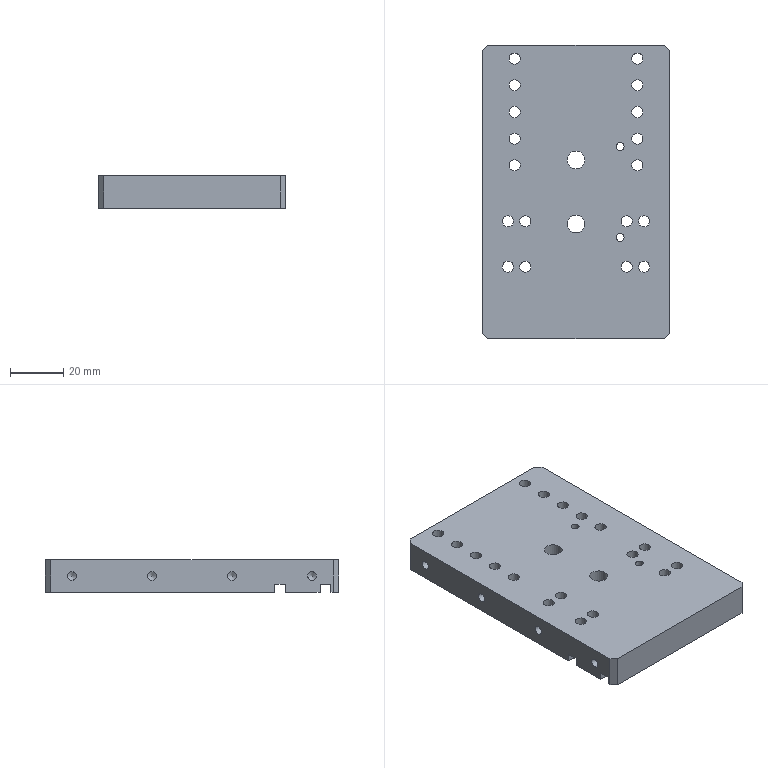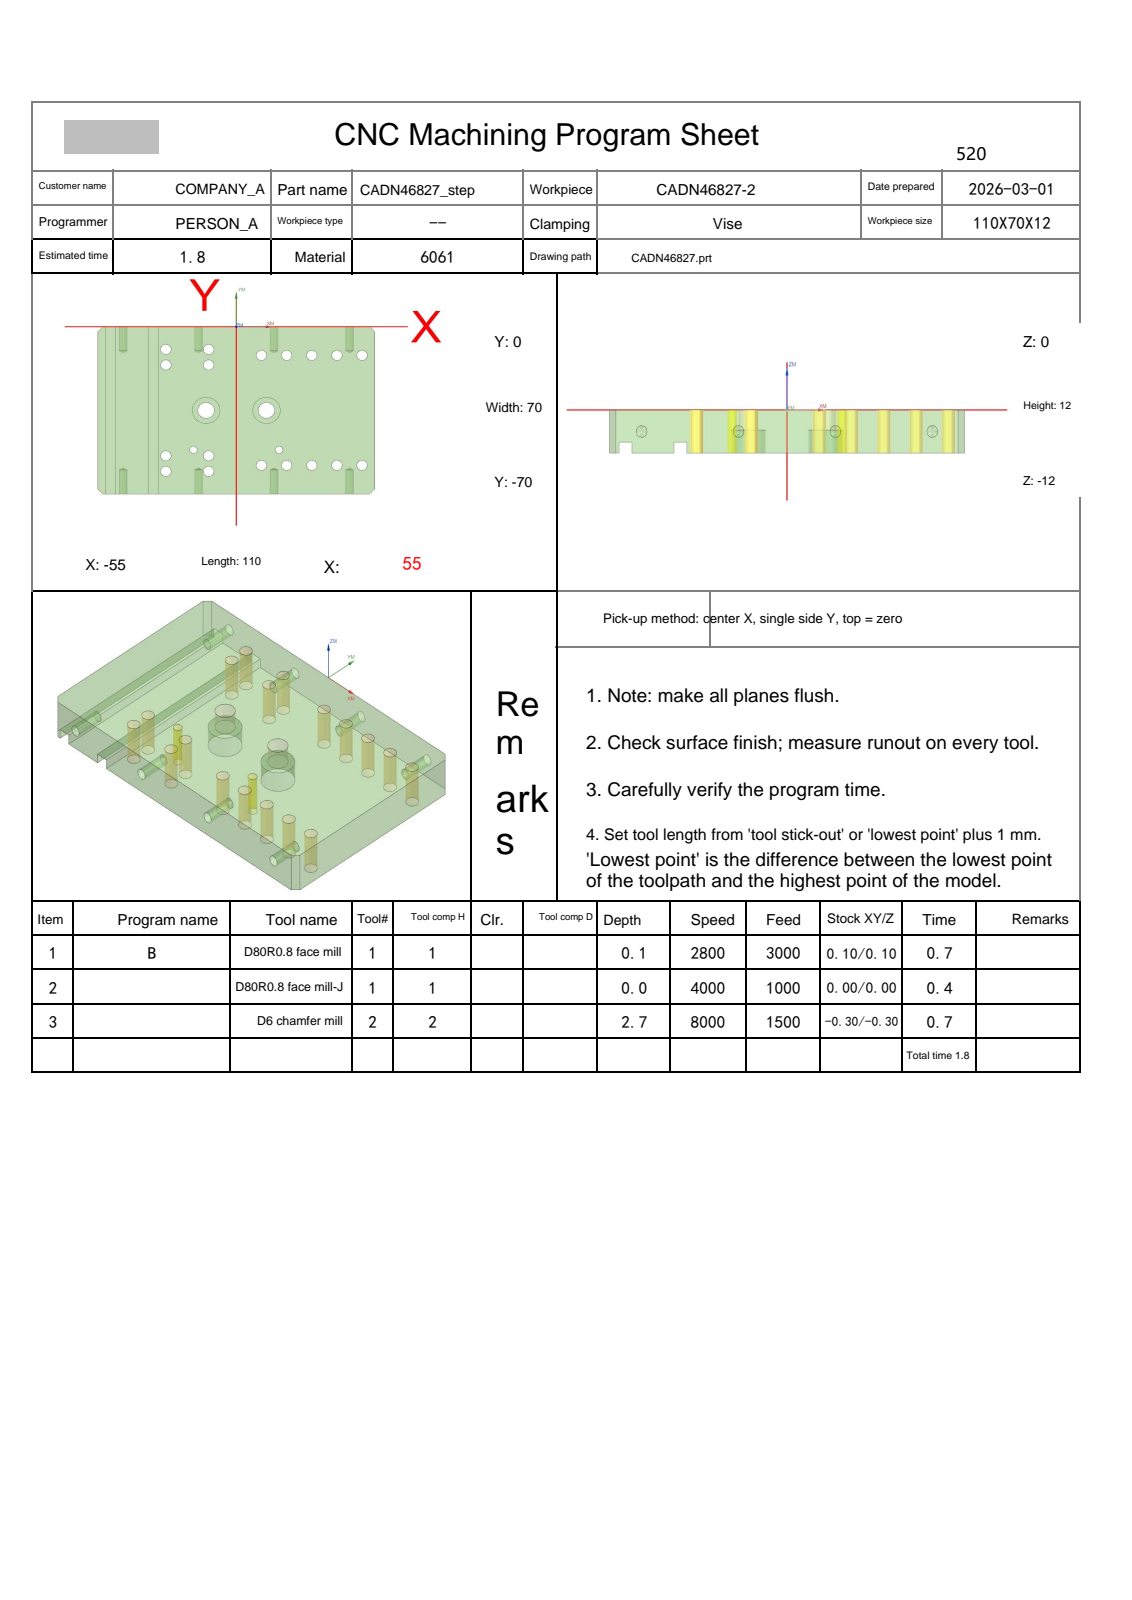NC program | NX | posted by the shop | part box 70 x 110 x 12 mm
Whole program:
%
O0001
(Machine time: 2.40 MIN)
(===Total Tool:2===)
(T1=D80R0.8 face mill D=80. R=0.8 D- H01 Z=0.    )
(T2=D6 chamfer mill D=6. R=0. D- H02 Z=-2.7  )
G80 G90 G17 G49 G40
G91 G28 Z0
M01
N1 T01 M06
(D80R0.8 face mill D=80. R=0.8 H=01 ce=0.10 di=0.10)
G00 G90 G54 X-107.097 Y-23.903 M03 S2800
G43 H01 Z50.
M08
Z4.02
G01 Z2.02 F3000.
X-95.097
X88.422
G02 X95.097 Y-30.578 I0.0 J-6.675
G01 Y-30.737
G02 X87.097 Y-38.737 I-8. J0.0
G01 X-95.097
X-107.097
Z4.02
G00 Y-23.903
Z3.54
G01 Z1.54
X-95.097
X88.422
G02 X95.097 Y-30.578 I0.0 J-6.675
G01 Y-30.737
G02 X87.097 Y-38.737 I-8. J0.0
G01 X-95.097
X-107.097
Z3.54
G00 Y-23.903
Z3.06
G01 Z1.06
X-95.097
X88.422
G02 X95.097 Y-30.578 I0.0 J-6.675
G01 Y-30.737
G02 X87.097 Y-38.737 I-8. J0.0
G01 X-95.097
X-107.097
Z3.06
G00 Y-23.903
Z2.58
G01 Z.58
X-95.097
X88.422
G02 X95.097 Y-30.578 I0.0 J-6.675
G01 Y-30.737
G02 X87.097 Y-38.737 I-8. J0.0
G01 X-95.097
X-107.097
Z2.58
G00 Y-23.903
Z2.1
G01 Z.1
X-95.097
X88.422
G02 X95.097 Y-30.578 I0.0 J-6.675
G01 Y-30.737
G02 X87.097 Y-38.737 I-8. J0.0
G01 X-95.097
X-107.097
Z2.1
G00 Z50.
G91 G28 Z0.0
M05
M09
G91 G28 Z0.0
M01
N2 T01 M06
(D80R0.8 face mill-J D=80. R=0.8 H=01 ce=0.00 di=0.00)
G00 G90 G54 X-106.999 Y-24.001 M03 S4000
G43 H01 Z50.
M08
Z2.
G01 Z0.0 F1000.
X-94.999
X88.412
G02 X94.999 Y-30.588 I0.0 J-6.587
G01 Y-30.639
G02 X86.999 Y-38.639 I-8. J0.0
G01 X-94.999
X-106.999
Z2.
G00 Z50.
G91 G28 Z0.0
M05
M09
G91 G28 Z0.0
M01
N3 T02 M06
(D6 chamfer mill D=6. R=0. H=02 ce=0.00 di=0.00)
G00 G90 G54 X-17. Y-51.5 M03 S8000
G43 H02 Z50.
M08
G98 G81 X-17. Y-51.5 Z-1.8 R3. F1000.
X17.
G80
G00 Z50.
G00 G90 X50. Y-12. M03 S8000
Z50.
G98 G81 X50. Y-12. Z-2.7 R3. F1000.
X40.
X30.
X20.
X10.
X-11. Y-16.
Y-9.5
X-28.
Y-16.
Y-54.
Y-60.5
X-11.
Y-54.
X10. Y-58.
X20.
X30.
X40.
X50.
G80
G00 Z50.
G00 G90 X-13.087 Y-35.507 M03 S8000
Z50.
Z-.9
G01 Z-1.4 F1200.
X-13.5 Y-35.7
G03 X-12. Y-37.2 I1.5 J0.0
X-9.8 Y-35. I0.0 J2.2
X-12. Y-32.8 I-2.2 J0.0
X-14.2 Y-35. I0.0 J-2.2
X-12. Y-37.2 I2.2 J0.0
X-10.5 Y-35.7 I0.0 J1.5
G01 X-10.913 Y-35.507
Z-.9
G00 Z50.
X10.913
Z-.9
G01 Z-1.4
X10.5 Y-35.7
G03 X12. Y-37.2 I1.5 J0.0
X14.2 Y-35. I0.0 J2.2
X12. Y-32.8 I-2.2 J0.0
X9.8 Y-35. I0.0 J-2.2
X12. Y-37.2 I2.2 J0.0
X13.5 Y-35.7 I0.0 J1.5
G01 X13.087 Y-35.507
Z-.9
G00 Z50.
G00 G90 X.386 Y-71.227 M03 S6500
Z50.
Z.172
G01 Z-1.2 F1500.
G03 X.1 Y-71.027 I-1.286 J-1.532
G01 X.054 Y-70.997
X0.0 Y-71.
X-53.
X-53.259 Y-70.966
X-53.5 Y-70.866
X-53.707 Y-70.707
X-55.707 Y-68.707
X-55.866 Y-68.5
X-55.966 Y-68.259
X-56. Y-68.
Y-2.
X-55.966 Y-1.741
X-55.866 Y-1.5
X-55.707 Y-1.293
X-53.707 Y.707
X-53.5 Y.866
X-53.259 Y.966
X-53. Y1.
X53.
X53.259 Y.966
X53.5 Y.866
X53.707 Y.707
X55.707 Y-1.293
X55.866 Y-1.5
X55.966 Y-1.741
X56. Y-2.
Y-68.
X55.966 Y-68.259
X55.866 Y-68.5
X55.707 Y-68.707
X53.707 Y-70.707
X53.5 Y-70.866
X53.259 Y-70.966
X53. Y-71.
X0.0
X-.054 Y-70.997
X-.1 Y-71.027
G03 X-.386 Y-71.227 I1. J-1.732
G01 Z.172
G00 Z10.
X-28.412 Y-61.426
Z.32
G01 Z-1.2
G03 X-28.103 Y-61.586 I1.075 J1.687
G01 X-28.054 Y-61.61
X-28. Y-61.6
G03 X-26.9 Y-60.5 I0.0 J1.1
X-28. Y-59.4 I-1.1 J0.0
X-29.1 Y-60.5 I0.0 J-1.1
X-28. Y-61.6 I1.1 J0.0
G01 X-27.946 Y-61.61
X-27.897 Y-61.586
G03 X-27.588 Y-61.426 I-.765 J1.848
G01 Z.32
G00 Z2.55
X-28.412 Y-54.926
Z.32
G01 Z-1.2
G03 X-28.103 Y-55.086 I1.075 J1.687
G01 X-28.054 Y-55.11
X-28. Y-55.1
G03 X-26.9 Y-54. I0.0 J1.1
X-28. Y-52.9 I-1.1 J0.0
X-29.1 Y-54. I0.0 J-1.1
X-28. Y-55.1 I1.1 J0.0
G01 X-27.946 Y-55.11
X-27.897 Y-55.086
G03 X-27.588 Y-54.926 I-.765 J1.848
G01 Z.32
G00 Z2.55
X-16.581 Y-51.156
Z.447
G01 Z-1.2
G03 X-16.897 Y-51.009 I-1. J-1.732
G01 X-16.947 Y-50.988
X-17. Y-51.
G03 X-17.5 Y-51.5 I0.0 J-.5
X-17. Y-52. I.5 J0.0
X-16.5 Y-51.5 I0.0 J.5
X-17. Y-51. I-.5 J0.0
G01 X-17.053 Y-50.988
X-17.103 Y-51.009
G03 X-17.419 Y-51.156 I.684 J-1.879
G01 Z.447
G00 Z2.55
X-11.412 Y-54.926
Z.32
G01 Z-1.2
G03 X-11.103 Y-55.086 I1.075 J1.687
G01 X-11.054 Y-55.11
X-11. Y-55.1
G03 X-9.9 Y-54. I0.0 J1.1
X-11. Y-52.9 I-1.1 J0.0
X-12.1 Y-54. I0.0 J-1.1
X-11. Y-55.1 I1.1 J0.0
G01 X-10.946 Y-55.11
X-10.897 Y-55.086
G03 X-10.588 Y-54.926 I-.765 J1.848
G01 Z.32
G00 Z2.55
X-11.412 Y-61.426
Z.32
G01 Z-1.2
G03 X-11.103 Y-61.586 I1.075 J1.687
G01 X-11.054 Y-61.61
X-11. Y-61.6
G03 X-9.9 Y-60.5 I0.0 J1.1
X-11. Y-59.4 I-1.1 J0.0
X-12.1 Y-60.5 I0.0 J-1.1
X-11. Y-61.6 I1.1 J0.0
G01 X-10.946 Y-61.61
X-10.897 Y-61.586
G03 X-10.588 Y-61.426 I-.765 J1.848
G01 Z.32
G00 Z10.
X9.588 Y-58.926
Z.32
G01 Z-1.2
G03 X9.897 Y-59.086 I1.075 J1.687
G01 X9.946 Y-59.11
X10. Y-59.1
G03 X11.1 Y-58. I0.0 J1.1
X10. Y-56.9 I-1.1 J0.0
X8.9 Y-58. I0.0 J-1.1
X10. Y-59.1 I1.1 J0.0
G01 X10.054 Y-59.11
X10.103 Y-59.086
G03 X10.412 Y-58.926 I-.765 J1.848
G01 Z.32
G00 Z2.55
X17.419 Y-51.156
Z.447
G01 Z-1.2
G03 X17.103 Y-51.009 I-1. J-1.732
G01 X17.053 Y-50.988
X17. Y-51.
G03 X16.5 Y-51.5 I0.0 J-.5
X17. Y-52. I.5 J0.0
X17.5 Y-51.5 I0.0 J.5
X17. Y-51. I-.5 J0.0
G01 X16.947 Y-50.988
X16.897 Y-51.009
G03 X16.581 Y-51.156 I.684 J-1.879
G01 Z.447
G00 Z2.55
X19.588 Y-58.926
Z.32
G01 Z-1.2
G03 X19.897 Y-59.086 I1.075 J1.687
G01 X19.946 Y-59.11
X20. Y-59.1
G03 X21.1 Y-58. I0.0 J1.1
X20. Y-56.9 I-1.1 J0.0
X18.9 Y-58. I0.0 J-1.1
X20. Y-59.1 I1.1 J0.0
G01 X20.054 Y-59.11
X20.103 Y-59.086
G03 X20.412 Y-58.926 I-.765 J1.848
G01 Z.32
G00 Z2.55
X29.588
Z.32
G01 Z-1.2
G03 X29.897 Y-59.086 I1.075 J1.687
G01 X29.946 Y-59.11
X30. Y-59.1
G03 X31.1 Y-58. I0.0 J1.1
X30. Y-56.9 I-1.1 J0.0
X28.9 Y-58. I0.0 J-1.1
X30. Y-59.1 I1.1 J0.0
G01 X30.054 Y-59.11
X30.103 Y-59.086
G03 X30.412 Y-58.926 I-.765 J1.848
G01 Z.32
G00 Z2.55
X39.588
Z.32
G01 Z-1.2
G03 X39.897 Y-59.086 I1.075 J1.687
G01 X39.946 Y-59.11
X40. Y-59.1
G03 X41.1 Y-58. I0.0 J1.1
X40. Y-56.9 I-1.1 J0.0
X38.9 Y-58. I0.0 J-1.1
X40. Y-59.1 I1.1 J0.0
G01 X40.054 Y-59.11
X40.103 Y-59.086
G03 X40.412 Y-58.926 I-.765 J1.848
G01 Z.32
G00 Z2.55
X49.588
Z.32
G01 Z-1.2
G03 X49.897 Y-59.086 I1.075 J1.687
G01 X49.946 Y-59.11
X50. Y-59.1
G03 X51.1 Y-58. I0.0 J1.1
X50. Y-56.9 I-1.1 J0.0
X48.9 Y-58. I0.0 J-1.1
X50. Y-59.1 I1.1 J0.0
G01 X50.054 Y-59.11
X50.103 Y-59.086
G03 X50.412 Y-58.926 I-.765 J1.848
G01 Z.32
G00 Z10.
X49.588 Y-12.926
Z.32
G01 Z-1.2
G03 X49.897 Y-13.086 I1.075 J1.687
G01 X49.946 Y-13.11
X50. Y-13.1
G03 X51.1 Y-12. I0.0 J1.1
X50. Y-10.9 I-1.1 J0.0
X48.9 Y-12. I0.0 J-1.1
X50. Y-13.1 I1.1 J0.0
G01 X50.054 Y-13.11
X50.103 Y-13.086
G03 X50.412 Y-12.926 I-.765 J1.848
G01 Z.32
G00 Z2.55
X39.588
Z.32
G01 Z-1.2
G03 X39.897 Y-13.086 I1.075 J1.687
G01 X39.946 Y-13.11
X40. Y-13.1
G03 X41.1 Y-12. I0.0 J1.1
X40. Y-10.9 I-1.1 J0.0
X38.9 Y-12. I0.0 J-1.1
X40. Y-13.1 I1.1 J0.0
G01 X40.054 Y-13.11
X40.103 Y-13.086
G03 X40.412 Y-12.926 I-.765 J1.848
G01 Z.32
G00 Z2.55
X29.588
Z.32
G01 Z-1.2
G03 X29.897 Y-13.086 I1.075 J1.687
G01 X29.946 Y-13.11
X30. Y-13.1
G03 X31.1 Y-12. I0.0 J1.1
X30. Y-10.9 I-1.1 J0.0
X28.9 Y-12. I0.0 J-1.1
X30. Y-13.1 I1.1 J0.0
G01 X30.054 Y-13.11
X30.103 Y-13.086
G03 X30.412 Y-12.926 I-.765 J1.848
G01 Z.32
G00 Z2.55
X19.588
Z.32
G01 Z-1.2
G03 X19.897 Y-13.086 I1.075 J1.687
G01 X19.946 Y-13.11
X20. Y-13.1
G03 X21.1 Y-12. I0.0 J1.1
X20. Y-10.9 I-1.1 J0.0
X18.9 Y-12. I0.0 J-1.1
X20. Y-13.1 I1.1 J0.0
G01 X20.054 Y-13.11
X20.103 Y-13.086
G03 X20.412 Y-12.926 I-.765 J1.848
G01 Z.32
G00 Z2.55
X9.588
Z.32
G01 Z-1.2
G03 X9.897 Y-13.086 I1.075 J1.687
G01 X9.946 Y-13.11
X10. Y-13.1
G03 X11.1 Y-12. I0.0 J1.1
X10. Y-10.9 I-1.1 J0.0
X8.9 Y-12. I0.0 J-1.1
X10. Y-13.1 I1.1 J0.0
G01 X10.054 Y-13.11
X10.103 Y-13.086
G03 X10.412 Y-12.926 I-.765 J1.848
G01 Z.32
G00 Z10.
X11.596 Y-37.108
Z.253
G01 Z-1.2
G03 X11.898 Y-37.282 I1.147 J1.638
G01 X11.946 Y-37.308
X12. Y-37.3
G03 X14.3 Y-35. I0.0 J2.3
X12. Y-32.7 I-2.3 J0.0
X9.7 Y-35. I0.0 J-2.3
X12. Y-37.3 I2.3 J0.0
G01 X12.054 Y-37.308
X12.102 Y-37.282
G03 X12.404 Y-37.108 I-.845 J1.813
G01 Z.253
G00 Z10.
X-12.404
Z.253
G01 Z-1.2
G03 X-12.102 Y-37.282 I1.147 J1.638
G01 X-12.054 Y-37.308
X-12. Y-37.3
G03 X-9.7 Y-35. I0.0 J2.3
X-12. Y-32.7 I-2.3 J0.0
X-14.3 Y-35. I0.0 J-2.3
X-12. Y-37.3 I2.3 J0.0
G01 X-11.946 Y-37.308
X-11.898 Y-37.282
G03 X-11.596 Y-37.108 I-.845 J1.813
G01 Z.253
G00 Z10.
X-11.412 Y-16.926
Z.32
G01 Z-1.2
G03 X-11.103 Y-17.086 I1.075 J1.687
G01 X-11.054 Y-17.11
X-11. Y-17.1
G03 X-9.9 Y-16. I0.0 J1.1
X-11. Y-14.9 I-1.1 J0.0
X-12.1 Y-16. I0.0 J-1.1
X-11. Y-17.1 I1.1 J0.0
G01 X-10.946 Y-17.11
X-10.897 Y-17.086
G03 X-10.588 Y-16.926 I-.765 J1.848
G01 Z.32
G00 Z2.55
X-11.412 Y-10.426
Z.32
G01 Z-1.2
G03 X-11.103 Y-10.586 I1.075 J1.687
G01 X-11.054 Y-10.61
X-11. Y-10.6
G03 X-9.9 Y-9.5 I0.0 J1.1
X-11. Y-8.4 I-1.1 J0.0
X-12.1 Y-9.5 I0.0 J-1.1
X-11. Y-10.6 I1.1 J0.0
G01 X-10.946 Y-10.61
X-10.897 Y-10.586
G03 X-10.588 Y-10.426 I-.765 J1.848
G01 Z.32
G00 Z10.
X-28.412
Z.32
G01 Z-1.2
G03 X-28.103 Y-10.586 I1.075 J1.687
G01 X-28.054 Y-10.61
X-28. Y-10.6
G03 X-26.9 Y-9.5 I0.0 J1.1
X-28. Y-8.4 I-1.1 J0.0
X-29.1 Y-9.5 I0.0 J-1.1
X-28. Y-10.6 I1.1 J0.0
G01 X-27.946 Y-10.61
X-27.897 Y-10.586
G03 X-27.588 Y-10.426 I-.765 J1.848
G01 Z.32
G00 Z2.55
X-28.412 Y-16.926
Z.32
G01 Z-1.2
G03 X-28.103 Y-17.086 I1.075 J1.687
G01 X-28.054 Y-17.11
X-28. Y-17.1
G03 X-26.9 Y-16. I0.0 J1.1
X-28. Y-14.9 I-1.1 J0.0
X-29.1 Y-16. I0.0 J-1.1
X-28. Y-17.1 I1.1 J0.0
G01 X-27.946 Y-17.11
X-27.897 Y-17.086
G03 X-27.588 Y-16.926 I-.765 J1.848
G01 Z.32
G00 Z50.
M05
M09
G91 G28 Z0.0
G91 G28 Y0.0
M30
%